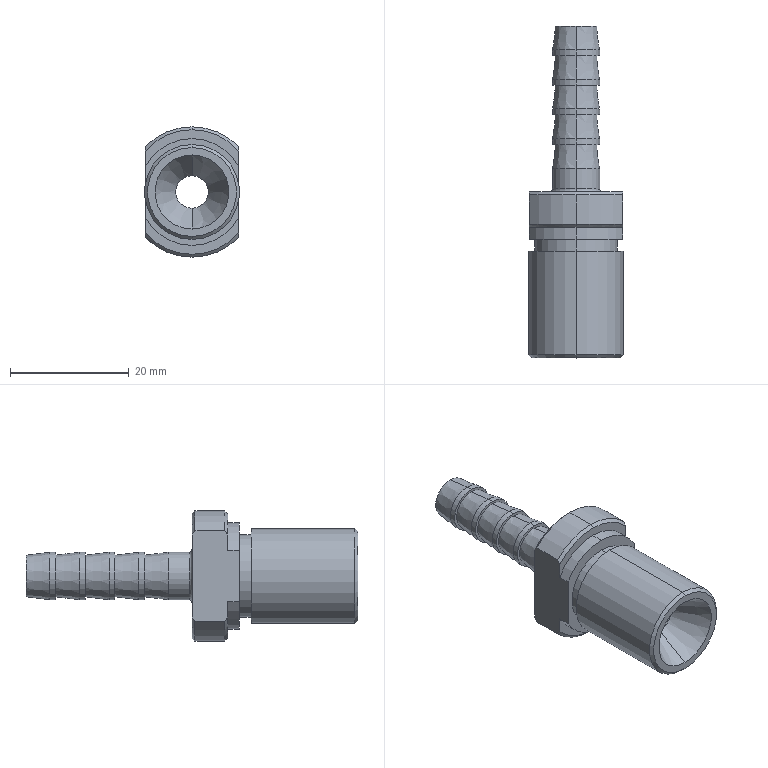Part | STEP file | HXGR200008-06-03-07 | 1 solid | 57 faces | box 16 x 56 x 22 mm | volume 5981 mm3 | cylinder 22 | cone 20 | plane 13 | torus 2 | commonest cylinder face diameters 8 x10 18 x3 22 x3 5.5 x2 14 x2 16 x2